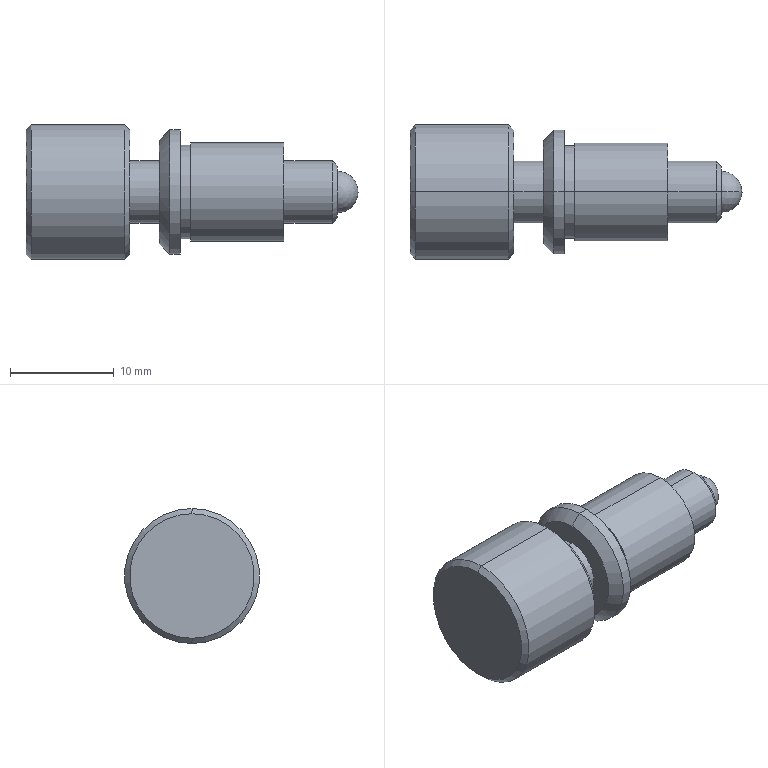Part | SolidWorks | features Revolution 1 | 1 solid | 29 faces | box 32 x 13 x 13 mm | volume 2468 mm3 | cylinder 12 | cone 8 | plane 7 | sphere 2 | commonest cylinder face diameters 6 x4 9 x2 9.5 x2 12 x2 13 x2
STEP:
#1=CARTESIAN_POINT('',(-15.546,0.,6.));
#2=VERTEX_POINT('',#1);
#3=CARTESIAN_POINT('',(-15.546,0.,-6.));
#4=VERTEX_POINT('',#3);
#5=CARTESIAN_POINT('',(-15.546,0.,0.));
#6=DIRECTION('',(-1.,0.,0.));
#7=DIRECTION('',(0.,0.,1.));
#8=AXIS2_PLACEMENT_3D('',#5,#6,#7);
#9=CIRCLE('',#8,6.);
#10=EDGE_CURVE('',#2,#4,#9,.T.);
#11=ORIENTED_EDGE('',*,*,#10,.F.);
#12=CARTESIAN_POINT('',(-15.046,0.,6.5));
#13=VERTEX_POINT('',#12);
#14=CARTESIAN_POINT('',(-15.046,0.,6.5));
#15=DIRECTION('',(0.7071,0.,0.7071));
#16=VECTOR('',#15,1000.);
#17=LINE('',#14,#16);
#18=EDGE_CURVE('',#2,#13,#17,.T.);
#19=ORIENTED_EDGE('',*,*,#18,.T.);
#20=CARTESIAN_POINT('',(-15.046,0.,-6.5));
#21=VERTEX_POINT('',#20);
#22=CARTESIAN_POINT('',(-15.046,0.,0.));
#23=DIRECTION('',(-1.,0.,0.));
#24=DIRECTION('',(0.,0.,1.));
#25=AXIS2_PLACEMENT_3D('',#22,#23,#24);
#26=CIRCLE('',#25,6.5);
#27=EDGE_CURVE('',#13,#21,#26,.T.);
#28=ORIENTED_EDGE('',*,*,#27,.T.);
#29=CARTESIAN_POINT('',(-15.046,0.,-6.5));
#30=DIRECTION('',(0.7071,0.,-0.7071));
#31=VECTOR('',#30,1000.);
#32=LINE('',#29,#31);
#33=EDGE_CURVE('',#4,#21,#32,.T.);
#34=ORIENTED_EDGE('',*,*,#33,.F.);
#35=EDGE_LOOP('',(#11,#19,#28,#34));
#36=FACE_OUTER_BOUND('',#35,.T.);
#37=CARTESIAN_POINT('',(-15.046,0.,0.));
#38=DIRECTION('',(1.,0.,0.));
#39=DIRECTION('',(0.,0.,-1.));
#40=AXIS2_PLACEMENT_3D('',#37,#38,#39);
#41=CONICAL_SURFACE('',#40,6.5,0.7854);
#42=ADVANCED_FACE('',(#36),#41,.T.);
#43=CARTESIAN_POINT('',(-6.046,0.,6.5));
#44=VERTEX_POINT('',#43);
#45=CARTESIAN_POINT('',(-6.046,0.,-6.5));
#46=VERTEX_POINT('',#45);
#47=CARTESIAN_POINT('',(-6.046,0.,0.));
#48=DIRECTION('',(-1.,0.,0.));
#49=DIRECTION('',(0.,0.,1.));
#50=AXIS2_PLACEMENT_3D('',#47,#48,#49);
#51=CIRCLE('',#50,6.5);
#52=EDGE_CURVE('',#44,#46,#51,.T.);
#53=ORIENTED_EDGE('',*,*,#52,.T.);
#54=CARTESIAN_POINT('',(-122.433,0.,-6.5));
#55=DIRECTION('',(-1.,0.,0.));
#56=VECTOR('',#55,1000.);
#57=LINE('',#54,#56);
#58=EDGE_CURVE('',#46,#21,#57,.T.);
#59=ORIENTED_EDGE('',*,*,#58,.T.);
#60=ORIENTED_EDGE('',*,*,#27,.F.);
#61=CARTESIAN_POINT('',(-122.433,0.,6.5));
#62=DIRECTION('',(-1.,0.,0.));
#63=VECTOR('',#62,1000.);
#64=LINE('',#61,#63);
#65=EDGE_CURVE('',#44,#13,#64,.T.);
#66=ORIENTED_EDGE('',*,*,#65,.F.);
#67=EDGE_LOOP('',(#53,#59,#60,#66));
#68=FACE_OUTER_BOUND('',#67,.T.);
#69=CARTESIAN_POINT('',(-122.433,0.,0.));
#70=DIRECTION('',(-1.,0.,0.));
#71=DIRECTION('',(0.,0.,1.));
#72=AXIS2_PLACEMENT_3D('',#69,#70,#71);
#73=CYLINDRICAL_SURFACE('',#72,6.5);
#74=ADVANCED_FACE('',(#68),#73,.T.);
#75=CARTESIAN_POINT('',(-5.546,0.,6.));
#76=VERTEX_POINT('',#75);
#77=CARTESIAN_POINT('',(-5.546,0.,-6.));
#78=VERTEX_POINT('',#77);
#79=CARTESIAN_POINT('',(-5.546,0.,0.));
#80=DIRECTION('',(-1.,0.,0.));
#81=DIRECTION('',(0.,0.,1.));
#82=AXIS2_PLACEMENT_3D('',#79,#80,#81);
#83=CIRCLE('',#82,6.);
#84=EDGE_CURVE('',#76,#78,#83,.T.);
#85=ORIENTED_EDGE('',*,*,#84,.T.);
#86=CARTESIAN_POINT('',(-5.546,0.,-6.));
#87=DIRECTION('',(-0.7071,0.,-0.7071));
#88=VECTOR('',#87,1000.);
#89=LINE('',#86,#88);
#90=EDGE_CURVE('',#78,#46,#89,.T.);
#91=ORIENTED_EDGE('',*,*,#90,.T.);
#92=ORIENTED_EDGE('',*,*,#52,.F.);
#93=CARTESIAN_POINT('',(-5.546,0.,6.));
#94=DIRECTION('',(-0.7071,0.,0.7071));
#95=VECTOR('',#94,1000.);
#96=LINE('',#93,#95);
#97=EDGE_CURVE('',#76,#44,#96,.T.);
#98=ORIENTED_EDGE('',*,*,#97,.F.);
#99=EDGE_LOOP('',(#85,#91,#92,#98));
#100=FACE_OUTER_BOUND('',#99,.T.);
#101=CARTESIAN_POINT('',(-5.546,0.,0.));
#102=DIRECTION('',(-1.,0.,0.));
#103=DIRECTION('',(0.,0.,1.));
#104=AXIS2_PLACEMENT_3D('',#101,#102,#103);
#105=CONICAL_SURFACE('',#104,6.,0.7854);
#106=ADVANCED_FACE('',(#100),#105,.T.);
#107=CARTESIAN_POINT('',(-2.68,0.,3.));
#108=VERTEX_POINT('',#107);
#109=CARTESIAN_POINT('',(-2.68,0.,-3.));
#110=VERTEX_POINT('',#109);
#111=CARTESIAN_POINT('',(-2.68,0.,0.));
#112=DIRECTION('',(-1.,0.,0.));
#113=DIRECTION('',(0.,0.,1.));
#114=AXIS2_PLACEMENT_3D('',#111,#112,#113);
#115=CIRCLE('',#114,3.);
#116=EDGE_CURVE('',#108,#110,#115,.T.);
#117=ORIENTED_EDGE('',*,*,#116,.T.);
#118=CARTESIAN_POINT('',(-5.546,0.,-3.));
#119=VERTEX_POINT('',#118);
#120=CARTESIAN_POINT('',(-122.433,0.,-3.));
#121=DIRECTION('',(-1.,0.,0.));
#122=VECTOR('',#121,1000.);
#123=LINE('',#120,#122);
#124=EDGE_CURVE('',#110,#119,#123,.T.);
#125=ORIENTED_EDGE('',*,*,#124,.T.);
#126=CARTESIAN_POINT('',(-5.546,0.,3.));
#127=VERTEX_POINT('',#126);
#128=CARTESIAN_POINT('',(-5.546,0.,0.));
#129=DIRECTION('',(-1.,0.,0.));
#130=DIRECTION('',(0.,0.,1.));
#131=AXIS2_PLACEMENT_3D('',#128,#129,#130);
#132=CIRCLE('',#131,3.);
#133=EDGE_CURVE('',#127,#119,#132,.T.);
#134=ORIENTED_EDGE('',*,*,#133,.F.);
#135=CARTESIAN_POINT('',(-122.433,0.,3.));
#136=DIRECTION('',(-1.,0.,0.));
#137=VECTOR('',#136,1000.);
#138=LINE('',#135,#137);
#139=EDGE_CURVE('',#108,#127,#138,.T.);
#140=ORIENTED_EDGE('',*,*,#139,.F.);
#141=EDGE_LOOP('',(#117,#125,#134,#140));
#142=FACE_OUTER_BOUND('',#141,.T.);
#143=CARTESIAN_POINT('',(-122.433,0.,0.));
#144=DIRECTION('',(-1.,0.,0.));
#145=DIRECTION('',(0.,0.,1.));
#146=AXIS2_PLACEMENT_3D('',#143,#144,#145);
#147=CYLINDRICAL_SURFACE('',#146,3.);
#148=ADVANCED_FACE('',(#142),#147,.T.);
#149=CARTESIAN_POINT('',(-2.68,0.,5.));
#150=VERTEX_POINT('',#149);
#151=CARTESIAN_POINT('',(-2.68,0.,-5.));
#152=VERTEX_POINT('',#151);
#153=CARTESIAN_POINT('',(-2.68,0.,0.));
#154=DIRECTION('',(-1.,0.,0.));
#155=DIRECTION('',(0.,0.,1.));
#156=AXIS2_PLACEMENT_3D('',#153,#154,#155);
#157=CIRCLE('',#156,5.);
#158=EDGE_CURVE('',#150,#152,#157,.T.);
#159=ORIENTED_EDGE('',*,*,#158,.F.);
#160=CARTESIAN_POINT('',(-1.68,0.,6.));
#161=VERTEX_POINT('',#160);
#162=CARTESIAN_POINT('',(-1.68,0.,6.));
#163=DIRECTION('',(0.7071,0.,0.7071));
#164=VECTOR('',#163,1000.);
#165=LINE('',#162,#164);
#166=EDGE_CURVE('',#150,#161,#165,.T.);
#167=ORIENTED_EDGE('',*,*,#166,.T.);
#168=CARTESIAN_POINT('',(-1.68,0.,-6.));
#169=VERTEX_POINT('',#168);
#170=CARTESIAN_POINT('',(-1.68,0.,0.));
#171=DIRECTION('',(-1.,0.,0.));
#172=DIRECTION('',(0.,0.,1.));
#173=AXIS2_PLACEMENT_3D('',#170,#171,#172);
#174=CIRCLE('',#173,6.);
#175=EDGE_CURVE('',#161,#169,#174,.T.);
#176=ORIENTED_EDGE('',*,*,#175,.T.);
#177=CARTESIAN_POINT('',(-1.68,0.,-6.));
#178=DIRECTION('',(0.7071,0.,-0.7071));
#179=VECTOR('',#178,1000.);
#180=LINE('',#177,#179);
#181=EDGE_CURVE('',#152,#169,#180,.T.);
#182=ORIENTED_EDGE('',*,*,#181,.F.);
#183=EDGE_LOOP('',(#159,#167,#176,#182));
#184=FACE_OUTER_BOUND('',#183,.T.);
#185=CARTESIAN_POINT('',(-1.68,0.,0.));
#186=DIRECTION('',(1.,0.,0.));
#187=DIRECTION('',(0.,0.,-1.));
#188=AXIS2_PLACEMENT_3D('',#185,#186,#187);
#189=CONICAL_SURFACE('',#188,6.,0.7854);
#190=ADVANCED_FACE('',(#184),#189,.T.);
#191=CARTESIAN_POINT('',(-0.6801,0.,6.));
#192=VERTEX_POINT('',#191);
#193=CARTESIAN_POINT('',(-0.6801,0.,-6.));
#194=VERTEX_POINT('',#193);
#195=CARTESIAN_POINT('',(-0.6801,0.,0.));
#196=DIRECTION('',(-1.,0.,0.));
#197=DIRECTION('',(0.,0.,1.));
#198=AXIS2_PLACEMENT_3D('',#195,#196,#197);
#199=CIRCLE('',#198,6.);
#200=EDGE_CURVE('',#192,#194,#199,.T.);
#201=ORIENTED_EDGE('',*,*,#200,.T.);
#202=CARTESIAN_POINT('',(-122.433,0.,-6.));
#203=DIRECTION('',(-1.,0.,0.));
#204=VECTOR('',#203,1000.);
#205=LINE('',#202,#204);
#206=EDGE_CURVE('',#194,#169,#205,.T.);
#207=ORIENTED_EDGE('',*,*,#206,.T.);
#208=ORIENTED_EDGE('',*,*,#175,.F.);
#209=CARTESIAN_POINT('',(-122.433,0.,6.));
#210=DIRECTION('',(-1.,0.,0.));
#211=VECTOR('',#210,1000.);
#212=LINE('',#209,#211);
#213=EDGE_CURVE('',#192,#161,#212,.T.);
#214=ORIENTED_EDGE('',*,*,#213,.F.);
#215=EDGE_LOOP('',(#201,#207,#208,#214));
#216=FACE_OUTER_BOUND('',#215,.T.);
#217=CARTESIAN_POINT('',(-122.433,0.,0.));
#218=DIRECTION('',(-1.,0.,0.));
#219=DIRECTION('',(0.,0.,1.));
#220=AXIS2_PLACEMENT_3D('',#217,#218,#219);
#221=CYLINDRICAL_SURFACE('',#220,6.);
#222=ADVANCED_FACE('',(#216),#221,.T.);
#223=CARTESIAN_POINT('',(0.3199,0.,4.5));
#224=VERTEX_POINT('',#223);
#225=CARTESIAN_POINT('',(0.3199,0.,-4.5));
#226=VERTEX_POINT('',#225);
#227=CARTESIAN_POINT('',(0.3199,0.,0.));
#228=DIRECTION('',(-1.,0.,0.));
#229=DIRECTION('',(0.,0.,1.));
#230=AXIS2_PLACEMENT_3D('',#227,#228,#229);
#231=CIRCLE('',#230,4.5);
#232=EDGE_CURVE('',#224,#226,#231,.T.);
#233=ORIENTED_EDGE('',*,*,#232,.T.);
#234=CARTESIAN_POINT('',(-0.6801,0.,-4.5));
#235=VERTEX_POINT('',#234);
#236=CARTESIAN_POINT('',(-122.433,0.,-4.5));
#237=DIRECTION('',(-1.,0.,0.));
#238=VECTOR('',#237,1000.);
#239=LINE('',#236,#238);
#240=EDGE_CURVE('',#226,#235,#239,.T.);
#241=ORIENTED_EDGE('',*,*,#240,.T.);
#242=CARTESIAN_POINT('',(-0.6801,0.,4.5));
#243=VERTEX_POINT('',#242);
#244=CARTESIAN_POINT('',(-0.6801,0.,0.));
#245=DIRECTION('',(-1.,0.,0.));
#246=DIRECTION('',(0.,0.,1.));
#247=AXIS2_PLACEMENT_3D('',#244,#245,#246);
#248=CIRCLE('',#247,4.5);
#249=EDGE_CURVE('',#243,#235,#248,.T.);
#250=ORIENTED_EDGE('',*,*,#249,.F.);
#251=CARTESIAN_POINT('',(-122.433,0.,4.5));
#252=DIRECTION('',(-1.,0.,0.));
#253=VECTOR('',#252,1000.);
#254=LINE('',#251,#253);
#255=EDGE_CURVE('',#224,#243,#254,.T.);
#256=ORIENTED_EDGE('',*,*,#255,.F.);
#257=EDGE_LOOP('',(#233,#241,#250,#256));
#258=FACE_OUTER_BOUND('',#257,.T.);
#259=CARTESIAN_POINT('',(-122.433,0.,0.));
#260=DIRECTION('',(-1.,0.,0.));
#261=DIRECTION('',(0.,0.,1.));
#262=AXIS2_PLACEMENT_3D('',#259,#260,#261);
#263=CYLINDRICAL_SURFACE('',#262,4.5);
#264=ADVANCED_FACE('',(#258),#263,.T.);
#265=CARTESIAN_POINT('',(9.32,0.,4.75));
#266=VERTEX_POINT('',#265);
#267=CARTESIAN_POINT('',(9.32,0.,-4.75));
#268=VERTEX_POINT('',#267);
#269=CARTESIAN_POINT('',(9.32,0.,0.));
#270=DIRECTION('',(-1.,0.,0.));
#271=DIRECTION('',(0.,0.,1.));
#272=AXIS2_PLACEMENT_3D('',#269,#270,#271);
#273=CIRCLE('',#272,4.75);
#274=EDGE_CURVE('',#266,#268,#273,.T.);
#275=ORIENTED_EDGE('',*,*,#274,.T.);
#276=CARTESIAN_POINT('',(0.3199,0.,-4.75));
#277=VERTEX_POINT('',#276);
#278=CARTESIAN_POINT('',(-122.433,0.,-4.75));
#279=DIRECTION('',(-1.,0.,0.));
#280=VECTOR('',#279,1000.);
#281=LINE('',#278,#280);
#282=EDGE_CURVE('',#268,#277,#281,.T.);
#283=ORIENTED_EDGE('',*,*,#282,.T.);
#284=CARTESIAN_POINT('',(0.3199,0.,4.75));
#285=VERTEX_POINT('',#284);
#286=CARTESIAN_POINT('',(0.3199,0.,0.));
#287=DIRECTION('',(-1.,0.,0.));
#288=DIRECTION('',(0.,0.,1.));
#289=AXIS2_PLACEMENT_3D('',#286,#287,#288);
#290=CIRCLE('',#289,4.75);
#291=EDGE_CURVE('',#285,#277,#290,.T.);
#292=ORIENTED_EDGE('',*,*,#291,.F.);
#293=CARTESIAN_POINT('',(-122.433,0.,4.75));
#294=DIRECTION('',(-1.,0.,0.));
#295=VECTOR('',#294,1000.);
#296=LINE('',#293,#295);
#297=EDGE_CURVE('',#266,#285,#296,.T.);
#298=ORIENTED_EDGE('',*,*,#297,.F.);
#299=EDGE_LOOP('',(#275,#283,#292,#298));
#300=FACE_OUTER_BOUND('',#299,.T.);
#301=CARTESIAN_POINT('',(-122.433,0.,0.));
#302=DIRECTION('',(-1.,0.,0.));
#303=DIRECTION('',(0.,0.,1.));
#304=AXIS2_PLACEMENT_3D('',#301,#302,#303);
#305=CYLINDRICAL_SURFACE('',#304,4.75);
#306=ADVANCED_FACE('',(#300),#305,.T.);
#307=CARTESIAN_POINT('',(13.954,0.,3.));
#308=VERTEX_POINT('',#307);
#309=CARTESIAN_POINT('',(13.954,0.,-3.));
#310=VERTEX_POINT('',#309);
#311=CARTESIAN_POINT('',(13.954,0.,0.));
#312=DIRECTION('',(-1.,0.,0.));
#313=DIRECTION('',(0.,0.,1.));
#314=AXIS2_PLACEMENT_3D('',#311,#312,#313);
#315=CIRCLE('',#314,3.);
#316=EDGE_CURVE('',#308,#310,#315,.T.);
#317=ORIENTED_EDGE('',*,*,#316,.T.);
#318=CARTESIAN_POINT('',(9.32,0.,-3.));
#319=VERTEX_POINT('',#318);
#320=CARTESIAN_POINT('',(-122.433,0.,-3.));
#321=DIRECTION('',(-1.,0.,0.));
#322=VECTOR('',#321,1000.);
#323=LINE('',#320,#322);
#324=EDGE_CURVE('',#310,#319,#323,.T.);
#325=ORIENTED_EDGE('',*,*,#324,.T.);
#326=CARTESIAN_POINT('',(9.32,0.,3.));
#327=VERTEX_POINT('',#326);
#328=CARTESIAN_POINT('',(9.32,0.,0.));
#329=DIRECTION('',(-1.,0.,0.));
#330=DIRECTION('',(0.,0.,1.));
#331=AXIS2_PLACEMENT_3D('',#328,#329,#330);
#332=CIRCLE('',#331,3.);
#333=EDGE_CURVE('',#327,#319,#332,.T.);
#334=ORIENTED_EDGE('',*,*,#333,.F.);
#335=CARTESIAN_POINT('',(-122.433,0.,3.));
#336=DIRECTION('',(-1.,0.,0.));
#337=VECTOR('',#336,1000.);
#338=LINE('',#335,#337);
#339=EDGE_CURVE('',#308,#327,#338,.T.);
#340=ORIENTED_EDGE('',*,*,#339,.F.);
#341=EDGE_LOOP('',(#317,#325,#334,#340));
#342=FACE_OUTER_BOUND('',#341,.T.);
#343=CARTESIAN_POINT('',(-122.433,0.,0.));
#344=DIRECTION('',(-1.,0.,0.));
#345=DIRECTION('',(0.,0.,1.));
#346=AXIS2_PLACEMENT_3D('',#343,#344,#345);
#347=CYLINDRICAL_SURFACE('',#346,3.);
#348=ADVANCED_FACE('',(#342),#347,.T.);
#349=CARTESIAN_POINT('',(14.454,0.,2.5));
#350=VERTEX_POINT('',#349);
#351=CARTESIAN_POINT('',(14.454,0.,-2.5));
#352=VERTEX_POINT('',#351);
#353=CARTESIAN_POINT('',(14.454,0.,0.));
#354=DIRECTION('',(-1.,0.,0.));
#355=DIRECTION('',(0.,0.,1.));
#356=AXIS2_PLACEMENT_3D('',#353,#354,#355);
#357=CIRCLE('',#356,2.5);
#358=EDGE_CURVE('',#350,#352,#357,.T.);
#359=ORIENTED_EDGE('',*,*,#358,.T.);
#360=CARTESIAN_POINT('',(14.454,0.,-2.5));
#361=DIRECTION('',(-0.7071,0.,-0.7071));
#362=VECTOR('',#361,1000.);
#363=LINE('',#360,#362);
#364=EDGE_CURVE('',#352,#310,#363,.T.);
#365=ORIENTED_EDGE('',*,*,#364,.T.);
#366=ORIENTED_EDGE('',*,*,#316,.F.);
#367=CARTESIAN_POINT('',(14.454,0.,2.5));
#368=DIRECTION('',(-0.7071,0.,0.7071));
#369=VECTOR('',#368,1000.);
#370=LINE('',#367,#369);
#371=EDGE_CURVE('',#350,#308,#370,.T.);
#372=ORIENTED_EDGE('',*,*,#371,.F.);
#373=EDGE_LOOP('',(#359,#365,#366,#372));
#374=FACE_OUTER_BOUND('',#373,.T.);
#375=CARTESIAN_POINT('',(14.454,0.,0.));
#376=DIRECTION('',(-1.,0.,0.));
#377=DIRECTION('',(0.,0.,1.));
#378=AXIS2_PLACEMENT_3D('',#375,#376,#377);
#379=CONICAL_SURFACE('',#378,2.5,0.7854);
#380=ADVANCED_FACE('',(#374),#379,.T.);
#381=CARTESIAN_POINT('',(16.454,0.,0.));
#382=VERTEX_POINT('',#381);
#383=CARTESIAN_POINT('',(14.454,0.,2.));
#384=VERTEX_POINT('',#383);
#385=CARTESIAN_POINT('',(14.454,0.,0.));
#386=DIRECTION('',(0.,-1.,0.));
#387=DIRECTION('',(0.,0.,-1.));
#388=AXIS2_PLACEMENT_3D('',#385,#386,#387);
#389=CIRCLE('',#388,2.);
#390=EDGE_CURVE('',#382,#384,#389,.T.);
#391=ORIENTED_EDGE('',*,*,#390,.F.);
#392=CARTESIAN_POINT('',(14.454,0.,-2.));
#393=VERTEX_POINT('',#392);
#394=CARTESIAN_POINT('',(14.454,0.,0.));
#395=DIRECTION('',(0.,1.,0.));
#396=DIRECTION('',(0.,0.,1.));
#397=AXIS2_PLACEMENT_3D('',#394,#395,#396);
#398=CIRCLE('',#397,2.);
#399=EDGE_CURVE('',#382,#393,#398,.T.);
#400=ORIENTED_EDGE('',*,*,#399,.T.);
#401=CARTESIAN_POINT('',(14.454,0.,0.));
#402=DIRECTION('',(-1.,0.,0.));
#403=DIRECTION('',(0.,0.,1.));
#404=AXIS2_PLACEMENT_3D('',#401,#402,#403);
#405=CIRCLE('',#404,2.);
#406=EDGE_CURVE('',#384,#393,#405,.T.);
#407=ORIENTED_EDGE('',*,*,#406,.F.);
#408=EDGE_LOOP('',(#391,#400,#407));
#409=FACE_OUTER_BOUND('',#408,.T.);
#410=CARTESIAN_POINT('',(14.454,0.,0.));
#411=DIRECTION('',(0.,1.,0.));
#412=DIRECTION('',(0.,0.,1.));
#413=AXIS2_PLACEMENT_3D('',#410,#411,#412);
#414=SPHERICAL_SURFACE('',#413,2.);
#415=ADVANCED_FACE('',(#409),#414,.T.);
#416=ORIENTED_EDGE('',*,*,#399,.F.);
#417=ORIENTED_EDGE('',*,*,#390,.T.);
#418=CARTESIAN_POINT('',(14.454,0.,0.));
#419=DIRECTION('',(-1.,0.,0.));
#420=DIRECTION('',(0.,0.,1.));
#421=AXIS2_PLACEMENT_3D('',#418,#419,#420);
#422=CIRCLE('',#421,2.);
#423=EDGE_CURVE('',#393,#384,#422,.T.);
#424=ORIENTED_EDGE('',*,*,#423,.F.);
#425=EDGE_LOOP('',(#416,#417,#424));
#426=FACE_OUTER_BOUND('',#425,.T.);
#427=CARTESIAN_POINT('',(14.454,0.,0.));
#428=DIRECTION('',(0.,1.,0.));
#429=DIRECTION('',(0.,0.,1.));
#430=AXIS2_PLACEMENT_3D('',#427,#428,#429);
#431=SPHERICAL_SURFACE('',#430,2.);
#432=ADVANCED_FACE('',(#426),#431,.T.);
#433=ORIENTED_EDGE('',*,*,#358,.F.);
#434=CARTESIAN_POINT('',(14.454,0.,0.));
#435=DIRECTION('',(-1.,0.,0.));
#436=DIRECTION('',(0.,0.,1.));
#437=AXIS2_PLACEMENT_3D('',#434,#435,#436);
#438=CIRCLE('',#437,2.5);
#439=EDGE_CURVE('',#352,#350,#438,.T.);
#440=ORIENTED_EDGE('',*,*,#439,.F.);
#441=EDGE_LOOP('',(#433,#440));
#442=FACE_OUTER_BOUND('',#441,.T.);
#443=ORIENTED_EDGE('',*,*,#406,.T.);
#444=ORIENTED_EDGE('',*,*,#423,.T.);
#445=EDGE_LOOP('',(#443,#444));
#446=FACE_BOUND('',#445,.T.);
#447=CARTESIAN_POINT('',(14.454,0.,-2.5));
#448=DIRECTION('',(-1.,0.,0.));
#449=DIRECTION('',(0.,0.,1.));
#450=AXIS2_PLACEMENT_3D('',#447,#448,#449);
#451=PLANE('',#450);
#452=ADVANCED_FACE('',(#442,#446),#451,.F.);
#453=ORIENTED_EDGE('',*,*,#364,.F.);
#454=ORIENTED_EDGE('',*,*,#439,.T.);
#455=ORIENTED_EDGE('',*,*,#371,.T.);
#456=CARTESIAN_POINT('',(13.954,0.,0.));
#457=DIRECTION('',(-1.,0.,0.));
#458=DIRECTION('',(0.,0.,1.));
#459=AXIS2_PLACEMENT_3D('',#456,#457,#458);
#460=CIRCLE('',#459,3.);
#461=EDGE_CURVE('',#310,#308,#460,.T.);
#462=ORIENTED_EDGE('',*,*,#461,.F.);
#463=EDGE_LOOP('',(#453,#454,#455,#462));
#464=FACE_OUTER_BOUND('',#463,.T.);
#465=CARTESIAN_POINT('',(14.454,0.,0.));
#466=DIRECTION('',(-1.,0.,0.));
#467=DIRECTION('',(0.,0.,1.));
#468=AXIS2_PLACEMENT_3D('',#465,#466,#467);
#469=CONICAL_SURFACE('',#468,2.5,0.7854);
#470=ADVANCED_FACE('',(#464),#469,.T.);
#471=ORIENTED_EDGE('',*,*,#324,.F.);
#472=ORIENTED_EDGE('',*,*,#461,.T.);
#473=ORIENTED_EDGE('',*,*,#339,.T.);
#474=CARTESIAN_POINT('',(9.32,0.,0.));
#475=DIRECTION('',(-1.,0.,0.));
#476=DIRECTION('',(0.,0.,1.));
#477=AXIS2_PLACEMENT_3D('',#474,#475,#476);
#478=CIRCLE('',#477,3.);
#479=EDGE_CURVE('',#319,#327,#478,.T.);
#480=ORIENTED_EDGE('',*,*,#479,.F.);
#481=EDGE_LOOP('',(#471,#472,#473,#480));
#482=FACE_OUTER_BOUND('',#481,.T.);
#483=CARTESIAN_POINT('',(-122.433,0.,0.));
#484=DIRECTION('',(-1.,0.,0.));
#485=DIRECTION('',(0.,0.,1.));
#486=AXIS2_PLACEMENT_3D('',#483,#484,#485);
#487=CYLINDRICAL_SURFACE('',#486,3.);
#488=ADVANCED_FACE('',(#482),#487,.T.);
#489=ORIENTED_EDGE('',*,*,#274,.F.);
#490=CARTESIAN_POINT('',(9.32,0.,0.));
#491=DIRECTION('',(-1.,0.,0.));
#492=DIRECTION('',(0.,0.,1.));
#493=AXIS2_PLACEMENT_3D('',#490,#491,#492);
#494=CIRCLE('',#493,4.75);
#495=EDGE_CURVE('',#268,#266,#494,.T.);
#496=ORIENTED_EDGE('',*,*,#495,.F.);
#497=EDGE_LOOP('',(#489,#496));
#498=FACE_OUTER_BOUND('',#497,.T.);
#499=ORIENTED_EDGE('',*,*,#333,.T.);
#500=ORIENTED_EDGE('',*,*,#479,.T.);
#501=EDGE_LOOP('',(#499,#500));
#502=FACE_BOUND('',#501,.T.);
#503=CARTESIAN_POINT('',(9.32,0.,-4.75));
#504=DIRECTION('',(-1.,0.,0.));
#505=DIRECTION('',(0.,0.,1.));
#506=AXIS2_PLACEMENT_3D('',#503,#504,#505);
#507=PLANE('',#506);
#508=ADVANCED_FACE('',(#498,#502),#507,.F.);
#509=ORIENTED_EDGE('',*,*,#282,.F.);
#510=ORIENTED_EDGE('',*,*,#495,.T.);
#511=ORIENTED_EDGE('',*,*,#297,.T.);
#512=CARTESIAN_POINT('',(0.3199,0.,0.));
#513=DIRECTION('',(-1.,0.,0.));
#514=DIRECTION('',(0.,0.,1.));
#515=AXIS2_PLACEMENT_3D('',#512,#513,#514);
#516=CIRCLE('',#515,4.75);
#517=EDGE_CURVE('',#277,#285,#516,.T.);
#518=ORIENTED_EDGE('',*,*,#517,.F.);
#519=EDGE_LOOP('',(#509,#510,#511,#518));
#520=FACE_OUTER_BOUND('',#519,.T.);
#521=CARTESIAN_POINT('',(-122.433,0.,0.));
#522=DIRECTION('',(-1.,0.,0.));
#523=DIRECTION('',(0.,0.,1.));
#524=AXIS2_PLACEMENT_3D('',#521,#522,#523);
#525=CYLINDRICAL_SURFACE('',#524,4.75);
#526=ADVANCED_FACE('',(#520),#525,.T.);
#527=ORIENTED_EDGE('',*,*,#232,.F.);
#528=CARTESIAN_POINT('',(0.3199,0.,0.));
#529=DIRECTION('',(-1.,0.,0.));
#530=DIRECTION('',(0.,0.,1.));
#531=AXIS2_PLACEMENT_3D('',#528,#529,#530);
#532=CIRCLE('',#531,4.5);
#533=EDGE_CURVE('',#226,#224,#532,.T.);
#534=ORIENTED_EDGE('',*,*,#533,.F.);
#535=EDGE_LOOP('',(#527,#534));
#536=FACE_BOUND('',#535,.T.);
#537=ORIENTED_EDGE('',*,*,#291,.T.);
#538=ORIENTED_EDGE('',*,*,#517,.T.);
#539=EDGE_LOOP('',(#537,#538));
#540=FACE_OUTER_BOUND('',#539,.T.);
#541=CARTESIAN_POINT('',(0.3199,0.,-4.5));
#542=DIRECTION('',(1.,0.,0.));
#543=DIRECTION('',(0.,0.,-1.));
#544=AXIS2_PLACEMENT_3D('',#541,#542,#543);
#545=PLANE('',#544);
#546=ADVANCED_FACE('',(#536,#540),#545,.F.);
#547=ORIENTED_EDGE('',*,*,#240,.F.);
#548=ORIENTED_EDGE('',*,*,#533,.T.);
#549=ORIENTED_EDGE('',*,*,#255,.T.);
#550=CARTESIAN_POINT('',(-0.6801,0.,0.));
#551=DIRECTION('',(-1.,0.,0.));
#552=DIRECTION('',(0.,0.,1.));
#553=AXIS2_PLACEMENT_3D('',#550,#551,#552);
#554=CIRCLE('',#553,4.5);
#555=EDGE_CURVE('',#235,#243,#554,.T.);
#556=ORIENTED_EDGE('',*,*,#555,.F.);
#557=EDGE_LOOP('',(#547,#548,#549,#556));
#558=FACE_OUTER_BOUND('',#557,.T.);
#559=CARTESIAN_POINT('',(-122.433,0.,0.));
#560=DIRECTION('',(-1.,0.,0.));
#561=DIRECTION('',(0.,0.,1.));
#562=AXIS2_PLACEMENT_3D('',#559,#560,#561);
#563=CYLINDRICAL_SURFACE('',#562,4.5);
#564=ADVANCED_FACE('',(#558),#563,.T.);
#565=ORIENTED_EDGE('',*,*,#200,.F.);
#566=CARTESIAN_POINT('',(-0.6801,0.,0.));
#567=DIRECTION('',(-1.,0.,0.));
#568=DIRECTION('',(0.,0.,1.));
#569=AXIS2_PLACEMENT_3D('',#566,#567,#568);
#570=CIRCLE('',#569,6.);
#571=EDGE_CURVE('',#194,#192,#570,.T.);
#572=ORIENTED_EDGE('',*,*,#571,.F.);
#573=EDGE_LOOP('',(#565,#572));
#574=FACE_OUTER_BOUND('',#573,.T.);
#575=ORIENTED_EDGE('',*,*,#249,.T.);
#576=ORIENTED_EDGE('',*,*,#555,.T.);
#577=EDGE_LOOP('',(#575,#576));
#578=FACE_BOUND('',#577,.T.);
#579=CARTESIAN_POINT('',(-0.6801,0.,-6.));
#580=DIRECTION('',(-1.,0.,0.));
#581=DIRECTION('',(0.,0.,1.));
#582=AXIS2_PLACEMENT_3D('',#579,#580,#581);
#583=PLANE('',#582);
#584=ADVANCED_FACE('',(#574,#578),#583,.F.);
#585=ORIENTED_EDGE('',*,*,#206,.F.);
#586=ORIENTED_EDGE('',*,*,#571,.T.);
#587=ORIENTED_EDGE('',*,*,#213,.T.);
#588=CARTESIAN_POINT('',(-1.68,0.,0.));
#589=DIRECTION('',(-1.,0.,0.));
#590=DIRECTION('',(0.,0.,1.));
#591=AXIS2_PLACEMENT_3D('',#588,#589,#590);
#592=CIRCLE('',#591,6.);
#593=EDGE_CURVE('',#169,#161,#592,.T.);
#594=ORIENTED_EDGE('',*,*,#593,.F.);
#595=EDGE_LOOP('',(#585,#586,#587,#594));
#596=FACE_OUTER_BOUND('',#595,.T.);
#597=CARTESIAN_POINT('',(-122.433,0.,0.));
#598=DIRECTION('',(-1.,0.,0.));
#599=DIRECTION('',(0.,0.,1.));
#600=AXIS2_PLACEMENT_3D('',#597,#598,#599);
#601=CYLINDRICAL_SURFACE('',#600,6.);
#602=ADVANCED_FACE('',(#596),#601,.T.);
#603=ORIENTED_EDGE('',*,*,#166,.F.);
#604=CARTESIAN_POINT('',(-2.68,0.,0.));
#605=DIRECTION('',(-1.,0.,0.));
#606=DIRECTION('',(0.,0.,1.));
#607=AXIS2_PLACEMENT_3D('',#604,#605,#606);
#608=CIRCLE('',#607,5.);
#609=EDGE_CURVE('',#152,#150,#608,.T.);
#610=ORIENTED_EDGE('',*,*,#609,.F.);
#611=ORIENTED_EDGE('',*,*,#181,.T.);
#612=ORIENTED_EDGE('',*,*,#593,.T.);
#613=EDGE_LOOP('',(#603,#610,#611,#612));
#614=FACE_OUTER_BOUND('',#613,.T.);
#615=CARTESIAN_POINT('',(-1.68,0.,0.));
#616=DIRECTION('',(1.,0.,0.));
#617=DIRECTION('',(0.,0.,-1.));
#618=AXIS2_PLACEMENT_3D('',#615,#616,#617);
#619=CONICAL_SURFACE('',#618,6.,0.7854);
#620=ADVANCED_FACE('',(#614),#619,.T.);
#621=ORIENTED_EDGE('',*,*,#116,.F.);
#622=CARTESIAN_POINT('',(-2.68,0.,0.));
#623=DIRECTION('',(-1.,0.,0.));
#624=DIRECTION('',(0.,0.,1.));
#625=AXIS2_PLACEMENT_3D('',#622,#623,#624);
#626=CIRCLE('',#625,3.);
#627=EDGE_CURVE('',#110,#108,#626,.T.);
#628=ORIENTED_EDGE('',*,*,#627,.F.);
#629=EDGE_LOOP('',(#621,#628));
#630=FACE_BOUND('',#629,.T.);
#631=ORIENTED_EDGE('',*,*,#609,.T.);
#632=ORIENTED_EDGE('',*,*,#158,.T.);
#633=EDGE_LOOP('',(#631,#632));
#634=FACE_OUTER_BOUND('',#633,.T.);
#635=CARTESIAN_POINT('',(-2.68,0.,-3.));
#636=DIRECTION('',(1.,0.,0.));
#637=DIRECTION('',(0.,0.,-1.));
#638=AXIS2_PLACEMENT_3D('',#635,#636,#637);
#639=PLANE('',#638);
#640=ADVANCED_FACE('',(#630,#634),#639,.F.);
#641=ORIENTED_EDGE('',*,*,#124,.F.);
#642=ORIENTED_EDGE('',*,*,#627,.T.);
#643=ORIENTED_EDGE('',*,*,#139,.T.);
#644=CARTESIAN_POINT('',(-5.546,0.,0.));
#645=DIRECTION('',(-1.,0.,0.));
#646=DIRECTION('',(0.,0.,1.));
#647=AXIS2_PLACEMENT_3D('',#644,#645,#646);
#648=CIRCLE('',#647,3.);
#649=EDGE_CURVE('',#119,#127,#648,.T.);
#650=ORIENTED_EDGE('',*,*,#649,.F.);
#651=EDGE_LOOP('',(#641,#642,#643,#650));
#652=FACE_OUTER_BOUND('',#651,.T.);
#653=CARTESIAN_POINT('',(-122.433,0.,0.));
#654=DIRECTION('',(-1.,0.,0.));
#655=DIRECTION('',(0.,0.,1.));
#656=AXIS2_PLACEMENT_3D('',#653,#654,#655);
#657=CYLINDRICAL_SURFACE('',#656,3.);
#658=ADVANCED_FACE('',(#652),#657,.T.);
#659=ORIENTED_EDGE('',*,*,#84,.F.);
#660=CARTESIAN_POINT('',(-5.546,0.,0.));
#661=DIRECTION('',(-1.,0.,0.));
#662=DIRECTION('',(0.,0.,1.));
#663=AXIS2_PLACEMENT_3D('',#660,#661,#662);
#664=CIRCLE('',#663,6.);
#665=EDGE_CURVE('',#78,#76,#664,.T.);
#666=ORIENTED_EDGE('',*,*,#665,.F.);
#667=EDGE_LOOP('',(#659,#666));
#668=FACE_OUTER_BOUND('',#667,.T.);
#669=ORIENTED_EDGE('',*,*,#133,.T.);
#670=ORIENTED_EDGE('',*,*,#649,.T.);
#671=EDGE_LOOP('',(#669,#670));
#672=FACE_BOUND('',#671,.T.);
#673=CARTESIAN_POINT('',(-5.546,0.,-6.));
#674=DIRECTION('',(-1.,0.,0.));
#675=DIRECTION('',(0.,0.,1.));
#676=AXIS2_PLACEMENT_3D('',#673,#674,#675);
#677=PLANE('',#676);
#678=ADVANCED_FACE('',(#668,#672),#677,.F.);
#679=ORIENTED_EDGE('',*,*,#90,.F.);
#680=ORIENTED_EDGE('',*,*,#665,.T.);
#681=ORIENTED_EDGE('',*,*,#97,.T.);
#682=CARTESIAN_POINT('',(-6.046,0.,0.));
#683=DIRECTION('',(-1.,0.,0.));
#684=DIRECTION('',(0.,0.,1.));
#685=AXIS2_PLACEMENT_3D('',#682,#683,#684);
#686=CIRCLE('',#685,6.5);
#687=EDGE_CURVE('',#46,#44,#686,.T.);
#688=ORIENTED_EDGE('',*,*,#687,.F.);
#689=EDGE_LOOP('',(#679,#680,#681,#688));
#690=FACE_OUTER_BOUND('',#689,.T.);
#691=CARTESIAN_POINT('',(-5.546,0.,0.));
#692=DIRECTION('',(-1.,0.,0.));
#693=DIRECTION('',(0.,0.,1.));
#694=AXIS2_PLACEMENT_3D('',#691,#692,#693);
#695=CONICAL_SURFACE('',#694,6.,0.7854);
#696=ADVANCED_FACE('',(#690),#695,.T.);
#697=ORIENTED_EDGE('',*,*,#58,.F.);
#698=ORIENTED_EDGE('',*,*,#687,.T.);
#699=ORIENTED_EDGE('',*,*,#65,.T.);
#700=CARTESIAN_POINT('',(-15.046,0.,0.));
#701=DIRECTION('',(-1.,0.,0.));
#702=DIRECTION('',(0.,0.,1.));
#703=AXIS2_PLACEMENT_3D('',#700,#701,#702);
#704=CIRCLE('',#703,6.5);
#705=EDGE_CURVE('',#21,#13,#704,.T.);
#706=ORIENTED_EDGE('',*,*,#705,.F.);
#707=EDGE_LOOP('',(#697,#698,#699,#706));
#708=FACE_OUTER_BOUND('',#707,.T.);
#709=CARTESIAN_POINT('',(-122.433,0.,0.));
#710=DIRECTION('',(-1.,0.,0.));
#711=DIRECTION('',(0.,0.,1.));
#712=AXIS2_PLACEMENT_3D('',#709,#710,#711);
#713=CYLINDRICAL_SURFACE('',#712,6.5);
#714=ADVANCED_FACE('',(#708),#713,.T.);
#715=ORIENTED_EDGE('',*,*,#18,.F.);
#716=CARTESIAN_POINT('',(-15.546,0.,0.));
#717=DIRECTION('',(-1.,0.,0.));
#718=DIRECTION('',(0.,0.,1.));
#719=AXIS2_PLACEMENT_3D('',#716,#717,#718);
#720=CIRCLE('',#719,6.);
#721=EDGE_CURVE('',#4,#2,#720,.T.);
#722=ORIENTED_EDGE('',*,*,#721,.F.);
#723=ORIENTED_EDGE('',*,*,#33,.T.);
#724=ORIENTED_EDGE('',*,*,#705,.T.);
#725=EDGE_LOOP('',(#715,#722,#723,#724));
#726=FACE_OUTER_BOUND('',#725,.T.);
#727=CARTESIAN_POINT('',(-15.046,0.,0.));
#728=DIRECTION('',(1.,0.,0.));
#729=DIRECTION('',(0.,0.,-1.));
#730=AXIS2_PLACEMENT_3D('',#727,#728,#729);
#731=CONICAL_SURFACE('',#730,6.5,0.7854);
#732=ADVANCED_FACE('',(#726),#731,.T.);
#733=ORIENTED_EDGE('',*,*,#721,.T.);
#734=ORIENTED_EDGE('',*,*,#10,.T.);
#735=EDGE_LOOP('',(#733,#734));
#736=FACE_OUTER_BOUND('',#735,.T.);
#737=CARTESIAN_POINT('',(-15.546,0.,0.));
#738=DIRECTION('',(1.,0.,0.));
#739=DIRECTION('',(0.,0.,-1.));
#740=AXIS2_PLACEMENT_3D('',#737,#738,#739);
#741=PLANE('',#740);
#742=ADVANCED_FACE('',(#736),#741,.F.);
#743=CLOSED_SHELL('',(#42,#74,#106,#148,#190,#222,#264,#306,#348,#380,#415,#432,#452,#470,#488,#508,#526,#546,#564,#584,#602,#620,#640,#658,#678,#696,#714,#732,#742));
#744=MANIFOLD_SOLID_BREP('',#743);
#745=CARTESIAN_POINT('',(0.,0.,0.));
#746=DIRECTION('',(0.,0.,1.));
#747=DIRECTION('',(1.,0.,0.));
#748=AXIS2_PLACEMENT_3D('',#745,#746,#747);
#749=(LENGTH_UNIT()NAMED_UNIT(*)SI_UNIT(.MILLI.,.METRE.));
#750=UNCERTAINTY_MEASURE_WITH_UNIT(LENGTH_MEASURE(0.00001),#749,'','');
#751=(NAMED_UNIT(*)PLANE_ANGLE_UNIT()SI_UNIT($,.RADIAN.));
#752=(NAMED_UNIT(*)SI_UNIT($,.STERADIAN.)SOLID_ANGLE_UNIT());
#753=(GEOMETRIC_REPRESENTATION_CONTEXT(3)GLOBAL_UNCERTAINTY_ASSIGNED_CONTEXT((#750))GLOBAL_UNIT_ASSIGNED_CONTEXT((#749,#751,#752))REPRESENTATION_CONTEXT('',''));
#754=ADVANCED_BREP_SHAPE_REPRESENTATION('',(#744,#748),#753);